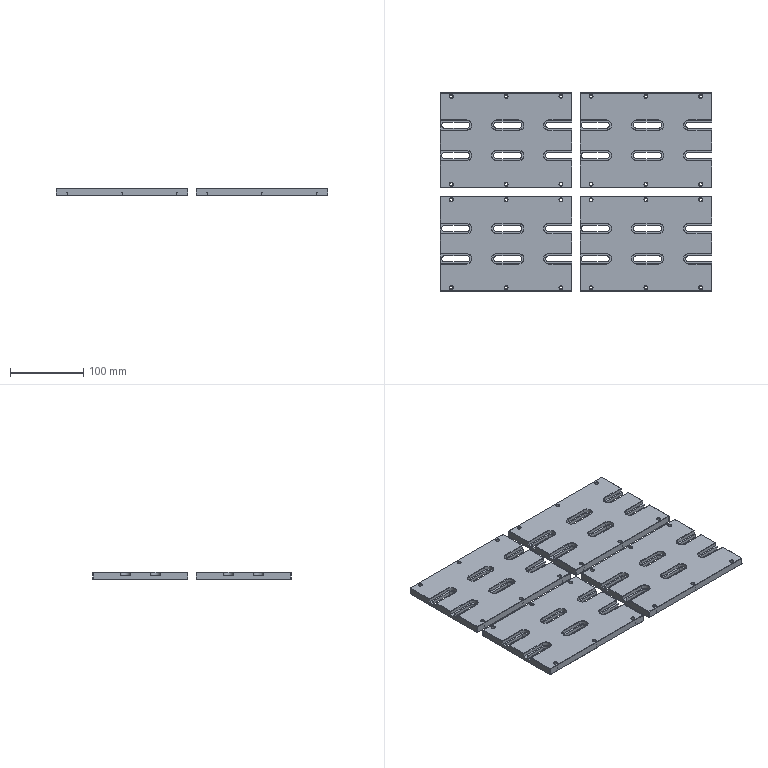Part | 4 solids | 744 faces | box 371 x 271 x 10 mm | volume 825733 mm3 | plane 328 | cone 232 | cylinder 184 | commonest cylinder face diameters 4.5 x48 8.1 x48 8.5 x40 13.5 x32 1 x16